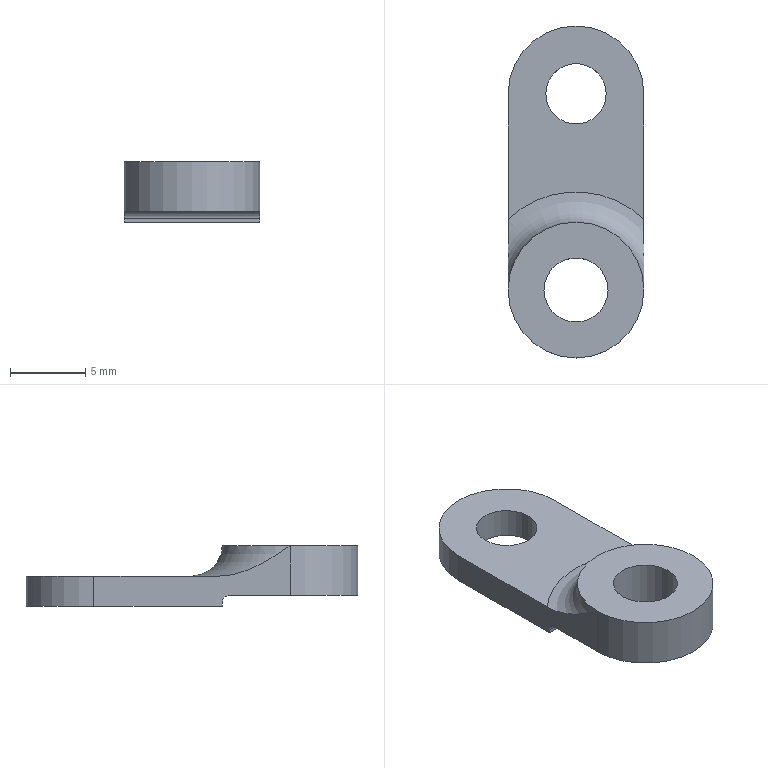CAM job | NX | 3-axis milling, drilling | part box 9 x 22 x 4 mm | stock box 17 x 35 x 8 mm
Tools:
number,name,description,diameter,corner_radius,flute_length,length,flutes
5,D4R0.5,Milling Tool-5 Parameters,4.0,0.5,50.0,75.0,2
4,D2-6-D4-50-3T-FINISH,D2-6-D4-50-3T-精,2.0,0.0,6.0,7.0,3
1,D10-30-D10-75-3T-FINISH,D10-30-D10-75-3T,10.0,0.0,30.0,75.0,3
3,钻头D3.8-48-76,钻刀D3.8-48-76,3.8,0.0,48.0,76.0,2
2,倒角D3-90度,倒角D3-90度,3.0,0.0,5.0,50.0,2
6,球刀R0.5-2-D4-50,球刀R0.5-2-D4-50,1.0,0.5,2.0,2.5,2
Operations:
program,operation,operation_type,tool,method,geometry_group,spindle_rpm,surface_speed,feed_per_tooth,feed_cut,feed_plunge,cut_length_mm,path_length_mm,cut_time_min,machine_time_min
A1,PLANAR_MILL,PlanarMilling,D10-30-D10-75-3T-FINISH,METHOD,WORKPIECE_54,3500.0,109.0,0.0762,800.0,100.0,48.0,82.0,0.06,0.0634
A1,ADAPTIVE_MILLING,CavityMilling,D10-30-D10-75-3T-FINISH,METHOD,WORKPIECE_54,4500.0,141.0,0.1481,2000.0,100.0,805.848,851.848,0.3713,0.3759
A1,PLANAR_MILL_1,PlanarMilling,D10-30-D10-75-3T-FINISH,METHOD,WORKPIECE_54,3500.0,109.0,0.0762,800.0,100.0,27.0,64.24,0.0337,0.0375
A1,DRILLING,Operation,倒角D3-90度,METHOD,WORKPIECE_54,3000.0,28.0,0.025,150.0,0.0,9.0,75.242,0.06,0.0666
A1,DRILLING_1,Operation,钻头D3.8-48-76,METHOD,WORKPIECE_54,3000.0,28.0,0.025,150.0,0.0,16.563,90.368,0.1104,0.1178
A1,HOLE_MILLING,CylinderMilling,D2-6-D4-50-3T-FINISH,METHOD,WORKPIECE_54,4500.0,28.0,0.0444,600.0,100.0,202.382,301.822,0.3373,0.3472
A1,HOLE_MILLING_COPY,CylinderMilling,D2-6-D4-50-3T-FINISH,METHOD,WORKPIECE_54,4500.0,28.0,0.0222,300.0,100.0,18.421,126.861,0.0614,0.0722
A1,PLANAR_MILL_2_COPY_COPY,PlanarMilling,D4R0.5,METHOD,WORKPIECE_54,4500.0,56.0,0.0889,800.0,100.0,84.0,284.361,0.105,0.125
A1,PLANAR_MILL_2_COPY,PlanarMilling,D4R0.5,METHOD,WORKPIECE_54,4500.0,56.0,0.0889,800.0,100.0,84.0,285.266,0.105,0.1251
A1,PLANAR_MILL_2,PlanarMilling,D4R0.5,METHOD,WORKPIECE_54,4500.0,56.0,0.0889,800.0,100.0,154.248,202.248,0.1928,0.1976
A1,PLANAR_MILL_3,PlanarMilling,球刀R0.5-2-D4-50,METHOD,WORKPIECE_54,4500.0,14.0,0.0889,800.0,100.0,49.792,86.192,0.0622,0.0659
A1,PLANAR_MILL_3_COPY,PlanarMilling,球刀R0.5-2-D4-50,METHOD,WORKPIECE_54,4500.0,14.0,0.0889,800.0,100.0,15.864,52.264,0.0198,0.0235
A1,PLANAR_MILL_3_COPY_1,PlanarMilling,球刀R0.5-2-D4-50,METHOD,WORKPIECE_54,4500.0,14.0,0.0889,800.0,100.0,27.022,64.862,0.0338,0.0376
A1,PLANAR_MILL_3_COPY_COPY,PlanarMilling,球刀R0.5-2-D4-50,METHOD,WORKPIECE_54,4500.0,14.0,0.0889,800.0,100.0,16.623,54.463,0.0208,0.0246
B1,ADAPTIVE_MILLING_1,CavityMilling,D10-30-D10-75-3T-FINISH,METHOD,WORKPIECE_55,4500.0,141.0,0.1111,1500.0,100.0,3145.944,3249.304,1.833,1.843
B1,FLOOR_WALL,VolumeBased25DMillingOperation,D4R0.5,METHOD,WORKPIECE_55,4500.0,56.0,0.0889,800.0,100.0,97.411,118.085,0.1218,0.1238
B1,PLANAR_MILL_4,PlanarMilling,D4R0.5,METHOD,WORKPIECE_55,4500.0,56.0,0.0889,800.0,100.0,32.892,32.892,0.0411,0.0411
B1,ZLEVEL_PROFILE_STEEP,ZLevelMilling,D4R0.5,METHOD,WORKPIECE_55,4500.0,56.0,0.1333,1200.0,100.0,612.116,612.116,0.5101,0.5101
B1,PLANAR_MILL_5,PlanarMilling,球刀R0.5-2-D4-50,METHOD,WORKPIECE_55,4500.0,14.0,0.0889,800.0,100.0,37.788,37.788,0.0472,0.0472
B1,PLANAR_MILL_5_COPY,PlanarMilling,球刀R0.5-2-D4-50,METHOD,WORKPIECE_55,4500.0,14.0,0.0889,800.0,100.0,19,19,0.0238,0.0238
B1,PLANAR_MILL_5_COPY_COPY,PlanarMilling,球刀R0.5-2-D4-50,METHOD,WORKPIECE_55,4500.0,14.0,0.0889,800.0,100.0,39.155,39.155,0.0489,0.0489